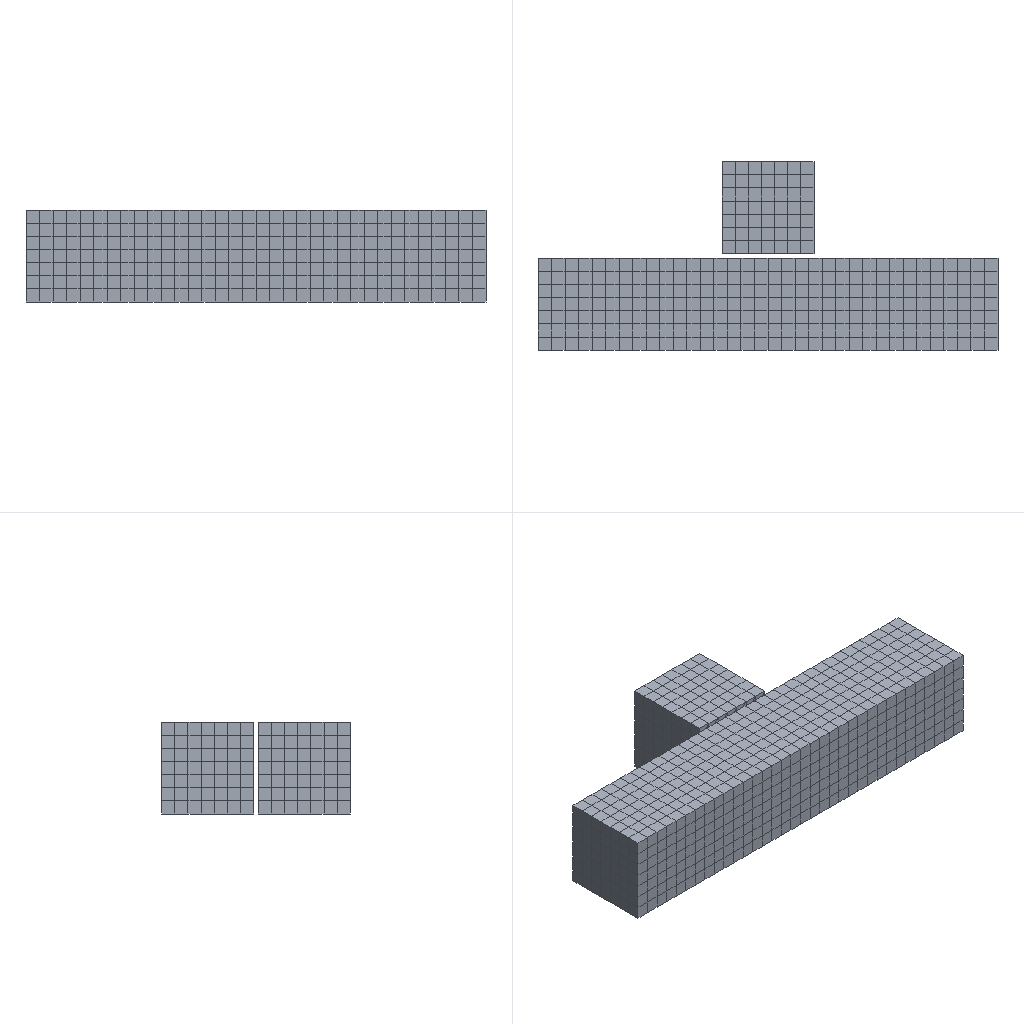Simulation study | ansys workbench
Set-up summary:
category,name,step,type,value,unit,region
solver,ansys_workbench
units,mm-N-s-tonne (MPa),,stated,"/units,MPA"
analysis,deck-1/LS1,,static
load_step,deck-1/LS1,deck-1/LS1,static,nsubst=1; time=1
analysis,deck-2/LS1,,static
load_step,deck-2/LS1,deck-2/LS1,static,nsubst=20; time=1
mesh,deck-1.dat,,nodes,10192
mesh,deck-1.dat,,elements,2632
element_type,SOLID186,,,2009,,deck-1.dat
element_type,TARGE170,,,287,,deck-1.dat
element_type,CONTA174,,,287,,deck-1.dat
element_type,SURF154,,,49,,deck-1.dat
mesh,deck-2.dat,,nodes,10192
mesh,deck-2.dat,,elements,2583
element_type,SOLID186,,,2009,,deck-2.dat
element_type,TARGE170,,,287,,deck-2.dat
element_type,CONTA174,,,287,,deck-2.dat
material,Structural Steel,,E,200000,tonne s^-2 mm^-1
material,Structural Steel,,nu,0.3
material,Structural Steel,,density,7.85e-09,tonne mm^-3
material,Structural Steel,,conductivity,60.5,tonne mm s^-3 C^-1
material,Structural Steel,,specific_heat,4.34e+08,mm^2 s^-2 C^-1
material,Structural Steel,,cte,1.2e-05,C^-1
material,Structural Steel,,permeability,10000
material,Structural Steel,,resistivity,0.00017,ohm mm
load,Define Pressure Vector Using Surface Effect Elements,deck-1/LS1,surface-effect pres face 2,-1,,SURF154 #5
bc,Fixed Supports,deck-1/model,fixed,[dofs=ALL],,_FIXEDSU
bc,Fixed Supports,deck-2/model,fixed,[dofs=ALL],,_FIXEDSU
bc,Constant Zero Displacement X,deck-2/model,fixed,[dofs=UX],,_DISPZEROUX
bc,Constant Zero Displacement Z,deck-2/model,fixed,[dofs=UZ],,_DISPZEROUZ
bc,Set Displacements,deck-2/LS1,prescribed uy,-600 [dofs=UY],,_CM59UY_YP
contact,Frictional - 2 To 1,,standard (frictionless/frictional),friction=0.15; element=CONTA174
contact,No Separation - 2 To 1,,no separation (always),element=CONTA174
named_set,_FIXEDSU,,node,352
named_set,_FIXEDSU,,node,352
named_set,_DISPZEROUX,,node,176
named_set,_DISPZEROUZ,,node,176
named_set,_CM59UY_YP,,node,176
Results summary:
result,analyses[0].index,,,1
result,analyses[0].system,,,SYS
result,analyses[0].deck,,,deck-1.dat
result,analyses[0].solve_status,,,completed
result,analyses[0].analysis_type,,,static
result,analyses[0].physics,,,mechanical
result,analyses[0].unit_system,,,"NMM: mm, ton, N, s, mV, mA, degC"
result,analyses[0].n_sets,,,1
result,analyses[0].load_steps[0].set,set=1,,1
result,analyses[0].load_steps[0].time_or_freq,set=1,,1
result,analyses[0].load_steps[0].max_displacement_magnitude,set=1,,0.5556
result,analyses[0].load_steps[0].max_von_mises_nodal,set=1,,4.969
result,analyses[0].load_steps[0].reaction_force_sum_xyz[1],set=1,,9.17804e-05
result,analyses[0].load_steps[0].reaction_force_sum_xyz[2],set=1,,1e+08
result,analyses[0].load_steps[0].reaction_force_sum_xyz[3],set=1,,-7.95486e-05
result,analyses[1].index,,,2
result,analyses[1].system,,,SYS-1
result,analyses[1].deck,,,deck-2.dat
result,analyses[1].solve_status,,,completed
result,analyses[1].analysis_type,,,static
result,analyses[1].physics,,,mechanical
result,analyses[1].unit_system,,,"NMM: mm, ton, N, s, mV, mA, degC"
result,analyses[1].n_sets,,,20
result,analyses[1].load_steps[0].set,set=20,,20
result,analyses[1].load_steps[0].time_or_freq,set=20,,1
result,analyses[1].load_steps[0].max_displacement_magnitude,set=20,,600
result,analyses[1].load_steps[0].max_von_mises_nodal,set=20,,895.533
result,analyses[1].load_steps[0].reaction_force_sum_xyz[1],set=20,,-15.779
result,analyses[1].load_steps[0].reaction_force_sum_xyz[2],set=20,,-2.415
result,analyses[1].load_steps[0].reaction_force_sum_xyz[3],set=20,,26.545
result,geometry_export[0][0],,,1.step
result,geometry_export[0][1],,,ok
result,geometry_export[0][2],,,2
result,geometry_export[1][0],,,2.step
result,geometry_export[1][1],,,ok
result,geometry_export[1][2],,,2